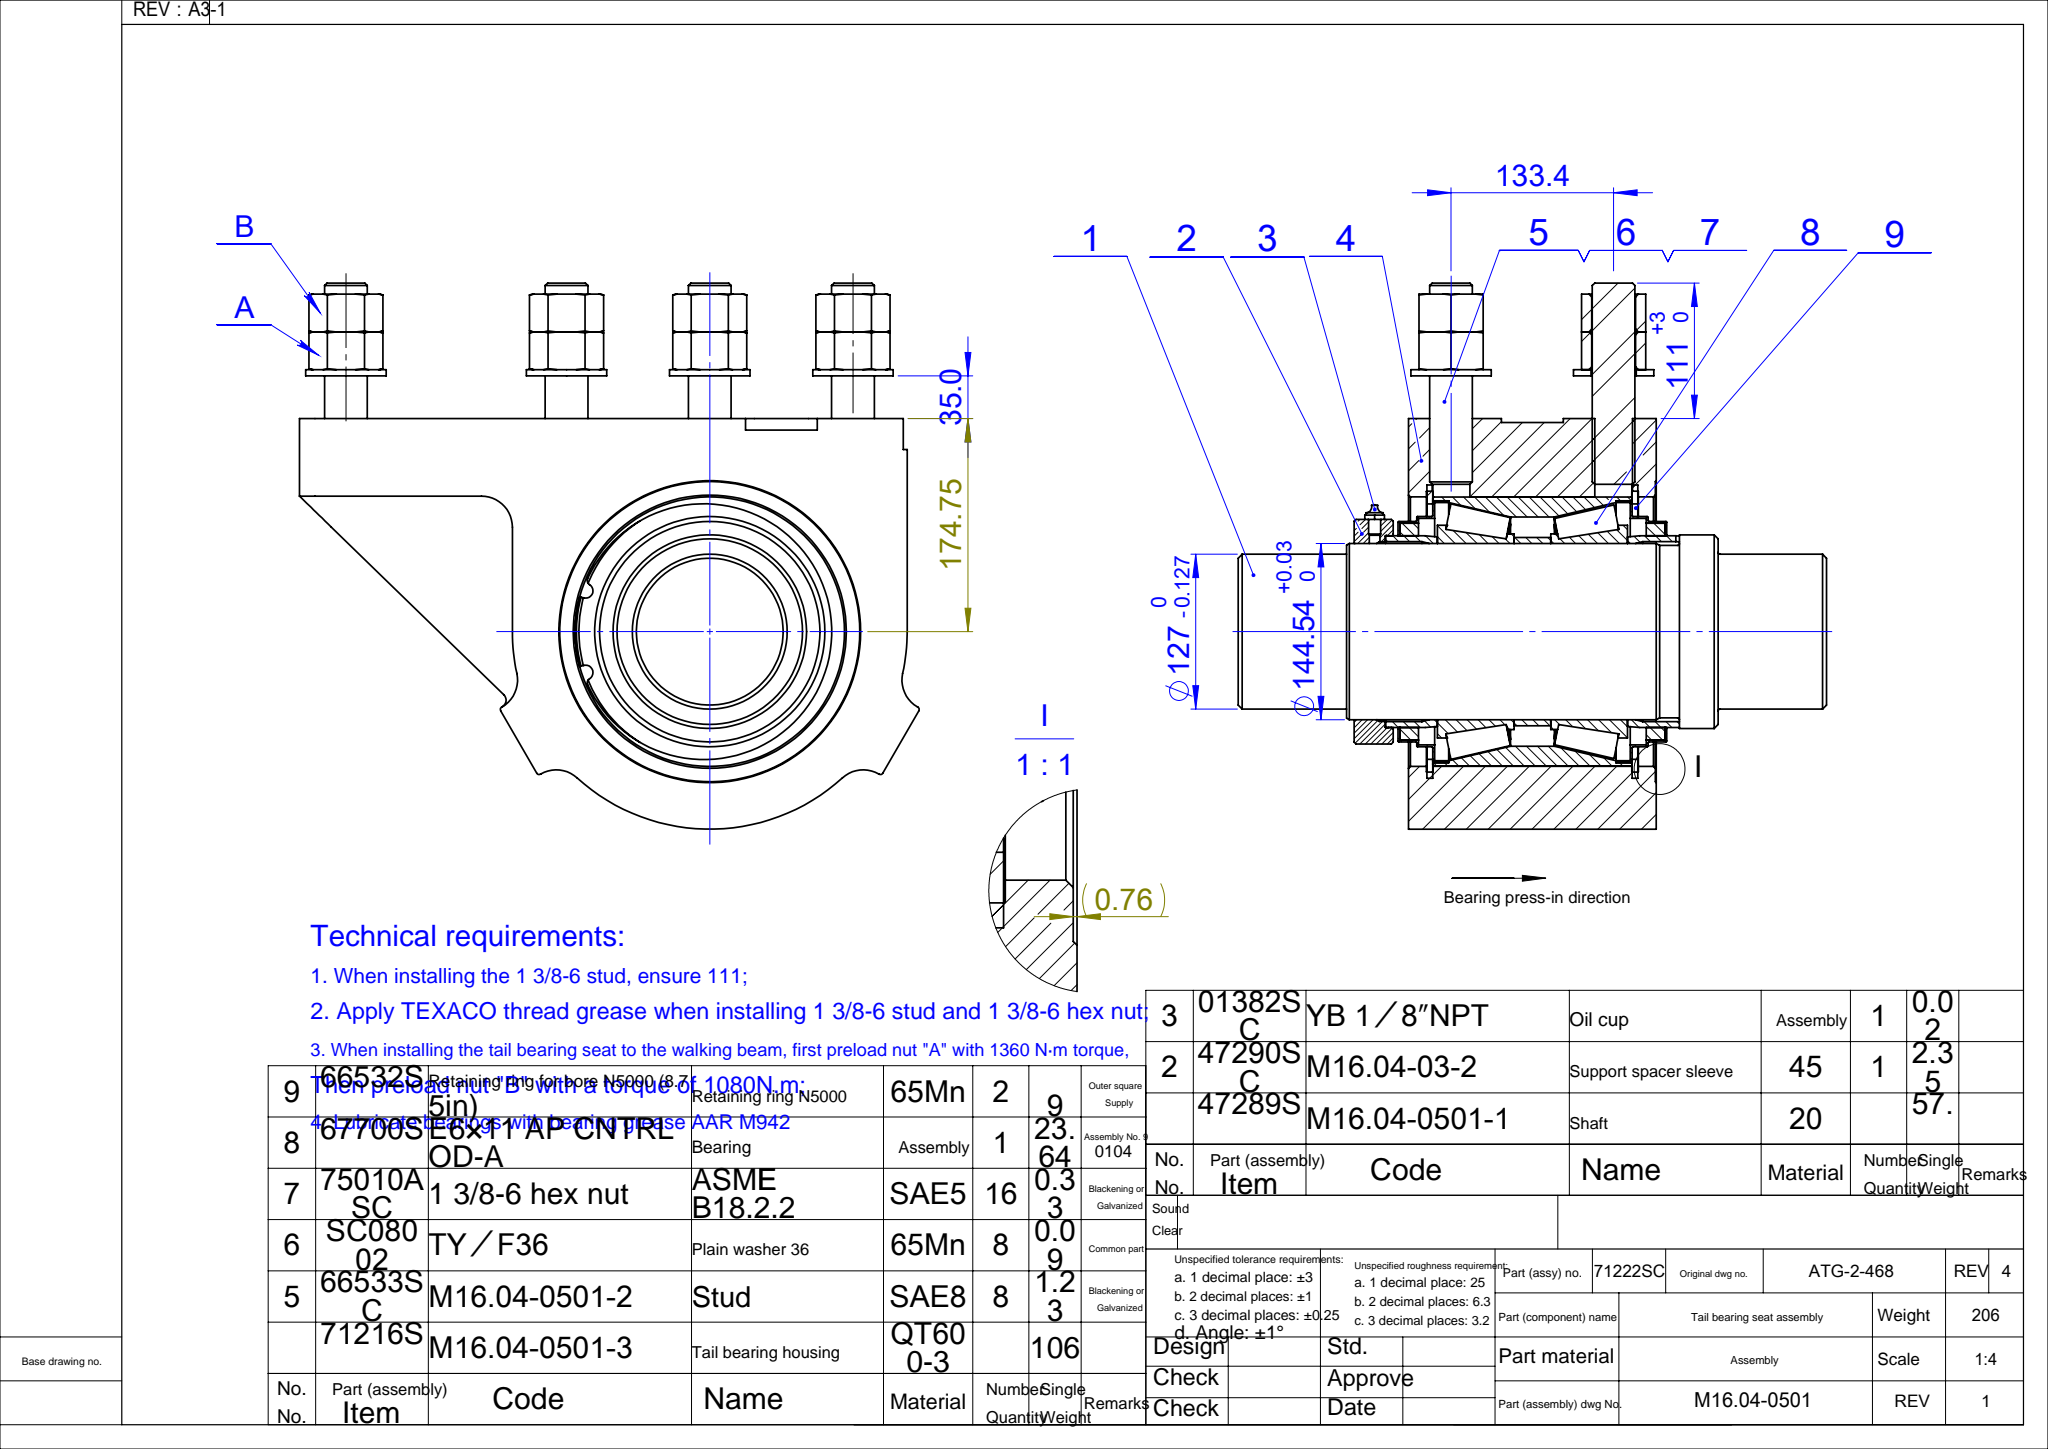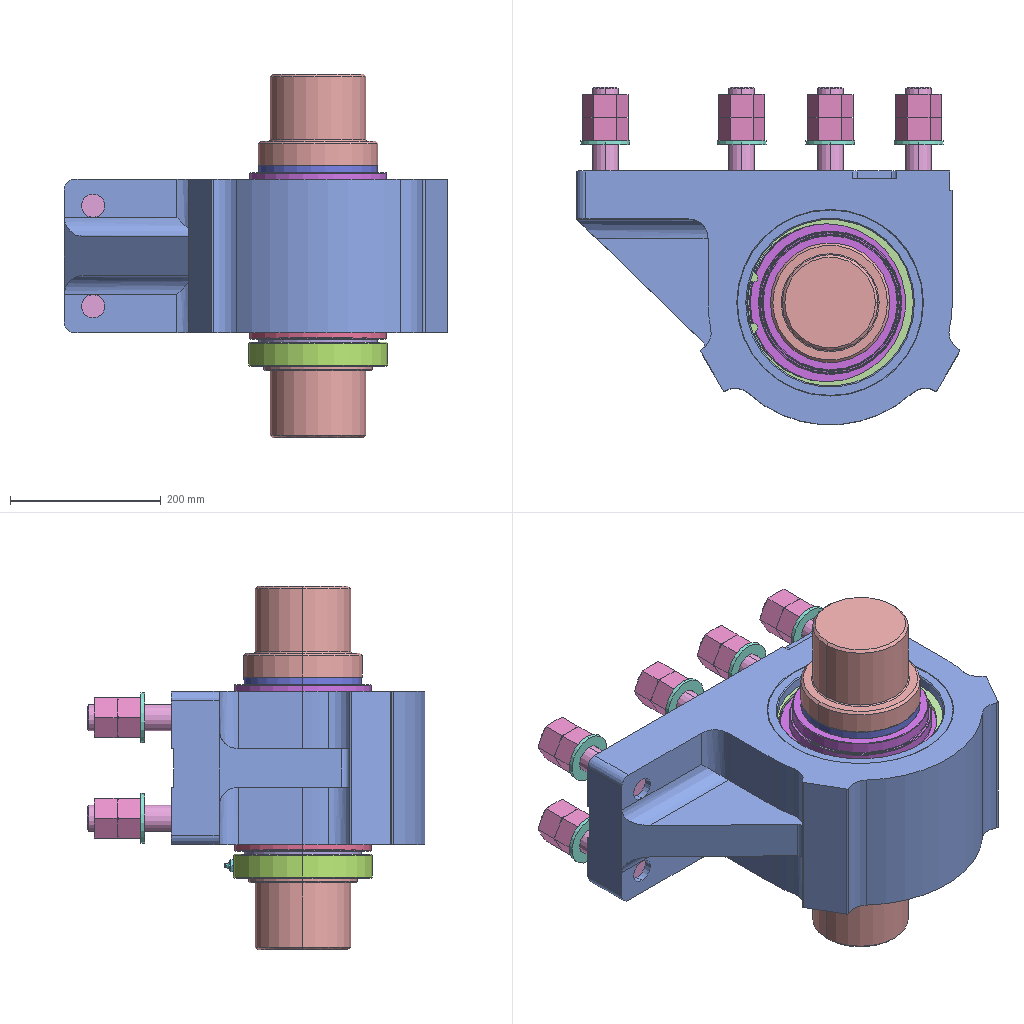Assembly | SolidWorks | 11 different items | 41 placed | box 508 x 447 x 483 mm
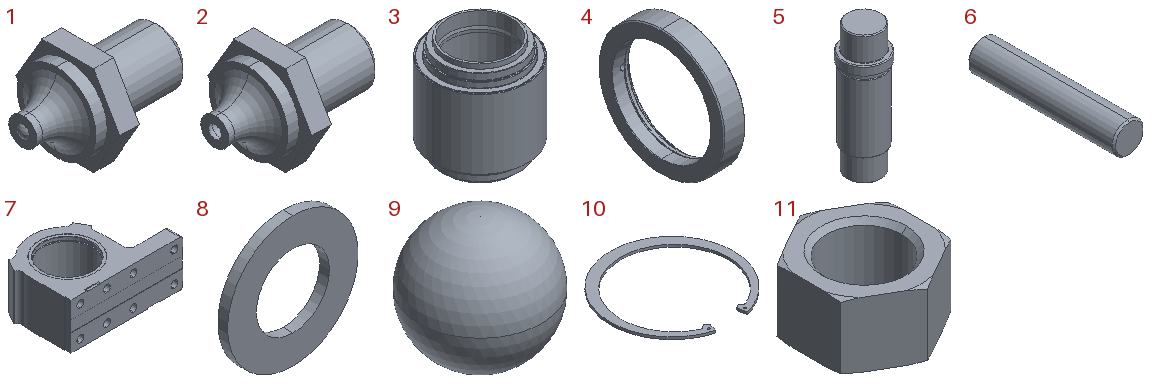Parts list (item | name | quantity | parent item | size | volume | features):
1 | (subassembly) | x1 | - | 25 x 18.475 x 16 mm | 2027 mm3 | -
2 | - | x1 | in 1 | 24.5 x 18.475 x 16 mm | 2013 mm3 | features RevCut 6, Revolution 2, Chamfer 1, Cut 1, Extrusion 1, Fillet 1, LPattern 1
3 | - | x1 | - | 220.662 x 220.662 x 241.2 mm | 3030333 mm3 | features Revolution 12, CirPattern 2, Fillet 2, Chamfer 1, Cut 1
4 | - | x1 | - | 32 x 184.15 x 184.15 mm | 301680 mm3 | features Chamfer 2, 3DProfileFeature 1, Cut 1, HoleWzd 1, Revolution 1
5 | - | x1 | - | 158.75 x 158.75 x 482.6 mm | 7340968 mm3 | features Revolution 1
6 | - | x8 | - | 35 x 165 x 35 mm | 158326 mm3 | features Chamfer 1, Revolution 1
7 | - | x1 | - | 508.317 x 336.677 x 203.2 mm | 15145778 mm3 | features Fillet 5, Cut 4, Boss 3, Chamfer 2, 3DProfileFeature 1, HoleWzd 1, RevCut 1, Revolution 1, Rib 1, SketchPattern 1
8 | - | x8 | - | 66 x 5 x 66 mm | 11730 mm3 | features Revolution 1
9 | - | x1 | in 1 | 3 x 3 x 3 mm | 14.137 mm3 | features Revolution 1
10 | - | x2 | - | 240.5 x 236.403 x 4.75 mm | 49385 mm3 | features Extrusion 1
11 | - | x16 | - | 52.765 x 60.79 x 31 mm | 42176 mm3 | features Cut 2, Chamfer 1, Extrusion 1
Mates (type | each side: item.copy, entity, surface, feature):
In the top assembly
Concentric | 5.1 face cylinder Revolve1 | 7.1 face cylinder Cut-Revolve1
Coincident | 7.1 plane | assembly plane
Concentric | 5.1 face cylinder Revolve1 | 4.1 face cylinder Revolve1
Coincident | 4.1 plane | assembly plane
Concentric | 7.1 face cylinder 1-3/8-6 Tapped Hole1 | 6.1 face cylinder Revolve1
DistanceDim | 6.1 face plane Revolve1 | 7.1 face plane Cut-Extrude3
Concentric | 6.1 face cylinder Revolve1 | 8.1 face cylinder Base-Revolve
DistanceDim | 8.1 face plane Base-Revolve | 7.1 face plane Cut-Extrude3
Concentric | 5.1 face cylinder Revolve1 | 3.1 face cylinder Revolve8
Coincident | 5.1 face plane Revolve1 | 3.1 face plane Revolve10
Coincident | 3.1 face plane Revolve3 | 4.1 face plane Revolve1
Coincident | 3.1 plane | assembly plane
Parallel | 7.1 face plane Revolve1 | 6.1 plane
Parallel | 7.1 face plane Revolve1 | 8.1 plane
Parallel | assembly plane | 7.1 face plane Cut-Extrude3
Concentric | 5.1 face cylinder Revolve1 | 10.1 face cylinder Base-Extrude
Concentric | 5.1 face cylinder Revolve1 | 10.2 face cylinder Base-Extrude
Concentric | 6.1 face cylinder Revolve1 | 11.1 face cylinder Base-Extrude
Coincident | 8.1 face plane Base-Revolve | 11.1 face plane Base-Extrude
Parallel | 7.1 face plane Revolve1 | 11.1 face plane Base-Extrude
Coincident | 3.1 face plane Revolve8 | 10.2 face plane Base-Extrude
Coincident | 3.1 face plane Revolve8 | 10.1 face plane Base-Extrude
Coincident | 10.2 plane | assembly plane
Coincident | 10.1 plane | assembly plane
Tangent | 4.1 face cylinder Revolve1 | 2.1 face plane Base-Extrude
Parallel | 4.1 face plane Revolve1 | 2.1 face plane Base-Extrude
Concentric | 6.1 face cylinder Revolve1 | 11.2 face cylinder Base-Extrude
Coincident | 11.1 face plane Base-Extrude | 11.2 face plane Base-Extrude | 2 times
In subassembly 1
Concentric | 2.2 face sphere Cut-Revolve6 | 9.1 face sphere Revolve1